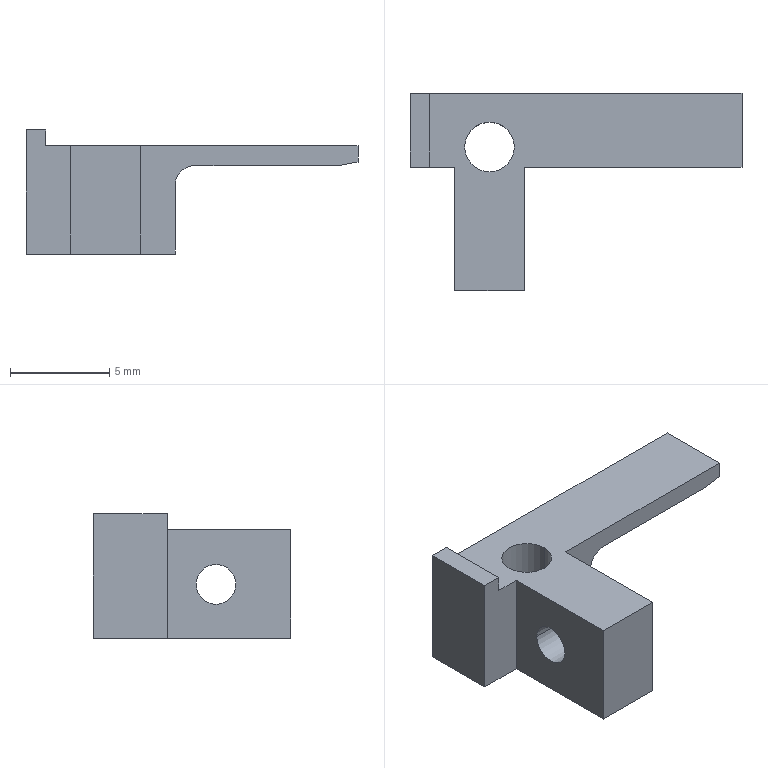Part | NX | 1 solid | 23 faces | box 16.7 x 9.913 x 6.24 mm | volume 257.778 mm3 | plane 16 | cylinder 7 | commonest cylinder face diameters 2 x3 2.5 x2 3.1 x2
STEP:
#1=CARTESIAN_POINT('',(-38.91,-45.316,4.443));
#2=VERTEX_POINT('',#1);
#3=CARTESIAN_POINT('',(-38.91,-45.316,3.629));
#4=VERTEX_POINT('',#3);
#5=CARTESIAN_POINT('',(-38.91,-45.316,4.403));
#6=DIRECTION('',(0.,0.,-1.));
#7=VECTOR('',#6,1000.);
#8=LINE('',#5,#7);
#9=EDGE_CURVE('',#2,#4,#8,.T.);
#10=ORIENTED_EDGE('',*,*,#9,.T.);
#11=CARTESIAN_POINT('',(-39.91,-45.316,3.453));
#12=VERTEX_POINT('',#11);
#13=CARTESIAN_POINT('',(-49.101,-45.316,1.833));
#14=DIRECTION('',(0.9848,0.,0.1736));
#15=VECTOR('',#14,1000.);
#16=LINE('',#13,#15);
#17=EDGE_CURVE('',#12,#4,#16,.T.);
#18=ORIENTED_EDGE('',*,*,#17,.F.);
#19=CARTESIAN_POINT('',(-47.11,-45.316,3.453));
#20=VERTEX_POINT('',#19);
#21=CARTESIAN_POINT('',(-49.101,-45.316,3.453));
#22=DIRECTION('',(-1.,0.,0.));
#23=VECTOR('',#22,1000.);
#24=LINE('',#21,#23);
#25=EDGE_CURVE('',#12,#20,#24,.T.);
#26=ORIENTED_EDGE('',*,*,#25,.T.);
#27=CARTESIAN_POINT('',(-48.11,-45.316,2.453));
#28=VERTEX_POINT('',#27);
#29=CARTESIAN_POINT('',(-47.11,-45.316,2.453));
#30=DIRECTION('',(0.,1.,0.));
#31=DIRECTION('',(0.,0.,1.));
#32=AXIS2_PLACEMENT_3D('',#29,#30,#31);
#33=CIRCLE('',#32,1.);
#34=EDGE_CURVE('',#28,#20,#33,.T.);
#35=ORIENTED_EDGE('',*,*,#34,.F.);
#36=CARTESIAN_POINT('',(-48.11,-45.316,-0.9969));
#37=VERTEX_POINT('',#36);
#38=CARTESIAN_POINT('',(-48.11,-45.316,4.403));
#39=DIRECTION('',(0.,0.,-1.));
#40=VECTOR('',#39,1000.);
#41=LINE('',#38,#40);
#42=EDGE_CURVE('',#28,#37,#41,.T.);
#43=ORIENTED_EDGE('',*,*,#42,.T.);
#44=CARTESIAN_POINT('',(-55.61,-45.316,-0.9969));
#45=VERTEX_POINT('',#44);
#46=CARTESIAN_POINT('',(-49.101,-45.316,-0.9969));
#47=DIRECTION('',(-1.,0.,0.));
#48=VECTOR('',#47,1000.);
#49=LINE('',#46,#48);
#50=EDGE_CURVE('',#37,#45,#49,.T.);
#51=ORIENTED_EDGE('',*,*,#50,.T.);
#52=CARTESIAN_POINT('',(-55.61,-45.316,5.243));
#53=VERTEX_POINT('',#52);
#54=CARTESIAN_POINT('',(-55.61,-45.316,4.403));
#55=DIRECTION('',(0.,0.,1.));
#56=VECTOR('',#55,1000.);
#57=LINE('',#54,#56);
#58=EDGE_CURVE('',#45,#53,#57,.T.);
#59=ORIENTED_EDGE('',*,*,#58,.T.);
#60=CARTESIAN_POINT('',(-54.61,-45.316,5.243));
#61=VERTEX_POINT('',#60);
#62=CARTESIAN_POINT('',(-49.101,-45.316,5.243));
#63=DIRECTION('',(1.,0.,0.));
#64=VECTOR('',#63,1000.);
#65=LINE('',#62,#64);
#66=EDGE_CURVE('',#53,#61,#65,.T.);
#67=ORIENTED_EDGE('',*,*,#66,.T.);
#68=CARTESIAN_POINT('',(-54.61,-45.316,4.443));
#69=VERTEX_POINT('',#68);
#70=CARTESIAN_POINT('',(-54.61,-45.316,4.403));
#71=DIRECTION('',(0.,0.,1.));
#72=VECTOR('',#71,1000.);
#73=LINE('',#70,#72);
#74=EDGE_CURVE('',#69,#61,#73,.T.);
#75=ORIENTED_EDGE('',*,*,#74,.F.);
#76=CARTESIAN_POINT('',(-49.101,-45.316,4.443));
#77=DIRECTION('',(1.,0.,0.));
#78=VECTOR('',#77,1000.);
#79=LINE('',#76,#78);
#80=EDGE_CURVE('',#69,#2,#79,.T.);
#81=ORIENTED_EDGE('',*,*,#80,.T.);
#82=EDGE_LOOP('',(#10,#18,#26,#35,#43,#51,#59,#67,#75,#81));
#83=FACE_BOUND('',#82,.T.);
#84=CARTESIAN_POINT('',(-43.64,-45.316,3.458));
#85=DIRECTION('',(0.,1.,0.));
#86=DIRECTION('',(1.,0.,0.));
#87=AXIS2_PLACEMENT_3D('',#84,#85,#86);
#88=PLANE('',#87);
#89=ADVANCED_FACE('',(#83),#88,.T.);
#90=CARTESIAN_POINT('',(-54.61,-49.029,5.243));
#91=VERTEX_POINT('',#90);
#92=CARTESIAN_POINT('',(-54.61,-49.029,4.443));
#93=VERTEX_POINT('',#92);
#94=CARTESIAN_POINT('',(-54.61,-49.029,4.403));
#95=DIRECTION('',(0.,0.,-1.));
#96=VECTOR('',#95,1000.);
#97=LINE('',#94,#96);
#98=EDGE_CURVE('',#91,#93,#97,.T.);
#99=ORIENTED_EDGE('',*,*,#98,.F.);
#100=CARTESIAN_POINT('',(-55.61,-49.029,5.243));
#101=VERTEX_POINT('',#100);
#102=CARTESIAN_POINT('',(-49.101,-49.029,5.243));
#103=DIRECTION('',(-1.,0.,0.));
#104=VECTOR('',#103,1000.);
#105=LINE('',#102,#104);
#106=EDGE_CURVE('',#91,#101,#105,.T.);
#107=ORIENTED_EDGE('',*,*,#106,.T.);
#108=CARTESIAN_POINT('',(-55.61,-49.029,-0.9969));
#109=VERTEX_POINT('',#108);
#110=CARTESIAN_POINT('',(-55.61,-49.029,4.403));
#111=DIRECTION('',(0.,0.,1.));
#112=VECTOR('',#111,1000.);
#113=LINE('',#110,#112);
#114=EDGE_CURVE('',#109,#101,#113,.T.);
#115=ORIENTED_EDGE('',*,*,#114,.F.);
#116=CARTESIAN_POINT('',(-53.36,-49.029,-0.9969));
#117=VERTEX_POINT('',#116);
#118=CARTESIAN_POINT('',(-49.101,-49.029,-0.9969));
#119=DIRECTION('',(-1.,0.,0.));
#120=VECTOR('',#119,1000.);
#121=LINE('',#118,#120);
#122=EDGE_CURVE('',#117,#109,#121,.T.);
#123=ORIENTED_EDGE('',*,*,#122,.F.);
#124=CARTESIAN_POINT('',(-53.36,-49.029,4.443));
#125=VERTEX_POINT('',#124);
#126=CARTESIAN_POINT('',(-53.36,-49.029,4.403));
#127=DIRECTION('',(0.,0.,1.));
#128=VECTOR('',#127,1000.);
#129=LINE('',#126,#128);
#130=EDGE_CURVE('',#117,#125,#129,.T.);
#131=ORIENTED_EDGE('',*,*,#130,.T.);
#132=CARTESIAN_POINT('',(-49.101,-49.029,4.443));
#133=DIRECTION('',(-1.,0.,0.));
#134=VECTOR('',#133,1000.);
#135=LINE('',#132,#134);
#136=EDGE_CURVE('',#125,#93,#135,.T.);
#137=ORIENTED_EDGE('',*,*,#136,.T.);
#138=EDGE_LOOP('',(#99,#107,#115,#123,#131,#137));
#139=FACE_BOUND('',#138,.T.);
#140=CARTESIAN_POINT('',(-54.61,-49.029,4.403));
#141=DIRECTION('',(0.,-1.,0.));
#142=DIRECTION('',(0.,0.,-1.));
#143=AXIS2_PLACEMENT_3D('',#140,#141,#142);
#144=PLANE('',#143);
#145=ADVANCED_FACE('',(#139),#144,.T.);
#146=CARTESIAN_POINT('',(-48.11,-49.029,2.453));
#147=VERTEX_POINT('',#146);
#148=CARTESIAN_POINT('',(-48.11,-51.163,2.453));
#149=DIRECTION('',(0.,1.,0.));
#150=VECTOR('',#149,1000.);
#151=LINE('',#148,#150);
#152=EDGE_CURVE('',#147,#28,#151,.T.);
#153=ORIENTED_EDGE('',*,*,#152,.F.);
#154=CARTESIAN_POINT('',(-48.11,-49.029,-0.9969));
#155=VERTEX_POINT('',#154);
#156=CARTESIAN_POINT('',(-48.11,-49.029,4.403));
#157=DIRECTION('',(0.,0.,1.));
#158=VECTOR('',#157,1000.);
#159=LINE('',#156,#158);
#160=EDGE_CURVE('',#155,#147,#159,.T.);
#161=ORIENTED_EDGE('',*,*,#160,.F.);
#162=CARTESIAN_POINT('',(-48.11,-51.163,-0.9969));
#163=DIRECTION('',(0.,-1.,0.));
#164=VECTOR('',#163,1000.);
#165=LINE('',#162,#164);
#166=EDGE_CURVE('',#37,#155,#165,.T.);
#167=ORIENTED_EDGE('',*,*,#166,.F.);
#168=ORIENTED_EDGE('',*,*,#42,.F.);
#169=EDGE_LOOP('',(#153,#161,#167,#168));
#170=FACE_BOUND('',#169,.T.);
#171=CARTESIAN_POINT('',(-48.11,-47.529,-0.5969));
#172=DIRECTION('',(1.,0.,0.));
#173=DIRECTION('',(0.,1.,0.));
#174=AXIS2_PLACEMENT_3D('',#171,#172,#173);
#175=PLANE('',#174);
#176=ADVANCED_FACE('',(#170),#175,.T.);
#177=CARTESIAN_POINT('',(-55.61,-51.163,5.243));
#178=DIRECTION('',(0.,1.,0.));
#179=VECTOR('',#178,1000.);
#180=LINE('',#177,#179);
#181=EDGE_CURVE('',#101,#53,#180,.T.);
#182=ORIENTED_EDGE('',*,*,#181,.F.);
#183=ORIENTED_EDGE('',*,*,#106,.F.);
#184=CARTESIAN_POINT('',(-54.61,-51.163,5.243));
#185=DIRECTION('',(0.,-1.,0.));
#186=VECTOR('',#185,1000.);
#187=LINE('',#184,#186);
#188=EDGE_CURVE('',#61,#91,#187,.T.);
#189=ORIENTED_EDGE('',*,*,#188,.F.);
#190=ORIENTED_EDGE('',*,*,#66,.F.);
#191=EDGE_LOOP('',(#182,#183,#189,#190));
#192=FACE_BOUND('',#191,.T.);
#193=CARTESIAN_POINT('',(-55.143,-49.311,5.243));
#194=DIRECTION('',(0.,0.,1.));
#195=DIRECTION('',(1.,0.,0.));
#196=AXIS2_PLACEMENT_3D('',#193,#194,#195);
#197=PLANE('',#196);
#198=ADVANCED_FACE('',(#192),#197,.T.);
#199=ORIENTED_EDGE('',*,*,#114,.T.);
#200=ORIENTED_EDGE('',*,*,#181,.T.);
#201=ORIENTED_EDGE('',*,*,#58,.F.);
#202=CARTESIAN_POINT('',(-55.61,-51.163,-0.9969));
#203=DIRECTION('',(0.,1.,0.));
#204=VECTOR('',#203,1000.);
#205=LINE('',#202,#204);
#206=EDGE_CURVE('',#109,#45,#205,.T.);
#207=ORIENTED_EDGE('',*,*,#206,.F.);
#208=EDGE_LOOP('',(#199,#200,#201,#207));
#209=FACE_BOUND('',#208,.T.);
#210=CARTESIAN_POINT('',(-55.61,-49.729,4.403));
#211=DIRECTION('',(-1.,0.,0.));
#212=DIRECTION('',(0.,0.,1.));
#213=AXIS2_PLACEMENT_3D('',#210,#211,#212);
#214=PLANE('',#213);
#215=ADVANCED_FACE('',(#209),#214,.T.);
#216=CARTESIAN_POINT('',(-54.61,-51.163,4.443));
#217=DIRECTION('',(0.,-1.,0.));
#218=VECTOR('',#217,1000.);
#219=LINE('',#216,#218);
#220=EDGE_CURVE('',#69,#93,#219,.T.);
#221=ORIENTED_EDGE('',*,*,#220,.F.);
#222=ORIENTED_EDGE('',*,*,#74,.T.);
#223=ORIENTED_EDGE('',*,*,#188,.T.);
#224=ORIENTED_EDGE('',*,*,#98,.T.);
#225=EDGE_LOOP('',(#221,#222,#223,#224));
#226=FACE_BOUND('',#225,.T.);
#227=CARTESIAN_POINT('',(-54.61,-45.316,4.403));
#228=DIRECTION('',(1.,0.,0.));
#229=DIRECTION('',(0.,1.,0.));
#230=AXIS2_PLACEMENT_3D('',#227,#228,#229);
#231=PLANE('',#230);
#232=ADVANCED_FACE('',(#226),#231,.T.);
#233=CARTESIAN_POINT('',(-38.91,-49.029,4.443));
#234=VERTEX_POINT('',#233);
#235=CARTESIAN_POINT('',(-38.91,-51.163,4.443));
#236=DIRECTION('',(0.,-1.,0.));
#237=VECTOR('',#236,1000.);
#238=LINE('',#235,#237);
#239=EDGE_CURVE('',#2,#234,#238,.T.);
#240=ORIENTED_EDGE('',*,*,#239,.F.);
#241=ORIENTED_EDGE('',*,*,#80,.F.);
#242=ORIENTED_EDGE('',*,*,#220,.T.);
#243=ORIENTED_EDGE('',*,*,#136,.F.);
#244=CARTESIAN_POINT('',(-53.36,-55.229,4.443));
#245=VERTEX_POINT('',#244);
#246=CARTESIAN_POINT('',(-53.36,-51.163,4.443));
#247=DIRECTION('',(0.,1.,0.));
#248=VECTOR('',#247,1000.);
#249=LINE('',#246,#248);
#250=EDGE_CURVE('',#245,#125,#249,.T.);
#251=ORIENTED_EDGE('',*,*,#250,.F.);
#252=CARTESIAN_POINT('',(-49.86,-55.229,4.443));
#253=VERTEX_POINT('',#252);
#254=CARTESIAN_POINT('',(-49.101,-55.229,4.443));
#255=DIRECTION('',(-1.,0.,0.));
#256=VECTOR('',#255,1000.);
#257=LINE('',#254,#256);
#258=EDGE_CURVE('',#253,#245,#257,.T.);
#259=ORIENTED_EDGE('',*,*,#258,.F.);
#260=CARTESIAN_POINT('',(-49.86,-49.029,4.443));
#261=VERTEX_POINT('',#260);
#262=CARTESIAN_POINT('',(-49.86,-51.163,4.443));
#263=DIRECTION('',(0.,-1.,0.));
#264=VECTOR('',#263,1000.);
#265=LINE('',#262,#264);
#266=EDGE_CURVE('',#261,#253,#265,.T.);
#267=ORIENTED_EDGE('',*,*,#266,.F.);
#268=CARTESIAN_POINT('',(-49.101,-49.029,4.443));
#269=DIRECTION('',(-1.,0.,0.));
#270=VECTOR('',#269,1000.);
#271=LINE('',#268,#270);
#272=EDGE_CURVE('',#234,#261,#271,.T.);
#273=ORIENTED_EDGE('',*,*,#272,.F.);
#274=EDGE_LOOP('',(#240,#241,#242,#243,#251,#259,#267,#273));
#275=FACE_BOUND('',#274,.T.);
#276=CARTESIAN_POINT('',(-50.36,-48.012,4.443));
#277=VERTEX_POINT('',#276);
#278=CARTESIAN_POINT('',(-52.86,-48.012,4.443));
#279=VERTEX_POINT('',#278);
#280=CARTESIAN_POINT('',(-51.61,-48.012,4.443));
#281=DIRECTION('',(0.,0.,-1.));
#282=DIRECTION('',(-1.,0.,0.));
#283=AXIS2_PLACEMENT_3D('',#280,#281,#282);
#284=CIRCLE('',#283,1.25);
#285=EDGE_CURVE('',#277,#279,#284,.T.);
#286=ORIENTED_EDGE('',*,*,#285,.T.);
#287=CARTESIAN_POINT('',(-51.61,-48.012,4.443));
#288=DIRECTION('',(0.,0.,-1.));
#289=DIRECTION('',(-1.,0.,0.));
#290=AXIS2_PLACEMENT_3D('',#287,#288,#289);
#291=CIRCLE('',#290,1.25);
#292=EDGE_CURVE('',#279,#277,#291,.T.);
#293=ORIENTED_EDGE('',*,*,#292,.T.);
#294=EDGE_LOOP('',(#286,#293));
#295=FACE_BOUND('',#294,.T.);
#296=CARTESIAN_POINT('',(-39.41,-47.687,4.443));
#297=DIRECTION('',(0.,0.,1.));
#298=DIRECTION('',(1.,0.,0.));
#299=AXIS2_PLACEMENT_3D('',#296,#297,#298);
#300=PLANE('',#299);
#301=ADVANCED_FACE('',(#275,#295),#300,.T.);
#302=CARTESIAN_POINT('',(-47.11,-49.029,3.453));
#303=VERTEX_POINT('',#302);
#304=CARTESIAN_POINT('',(-39.91,-49.029,3.453));
#305=VERTEX_POINT('',#304);
#306=CARTESIAN_POINT('',(-49.101,-49.029,3.453));
#307=DIRECTION('',(1.,0.,0.));
#308=VECTOR('',#307,1000.);
#309=LINE('',#306,#308);
#310=EDGE_CURVE('',#303,#305,#309,.T.);
#311=ORIENTED_EDGE('',*,*,#310,.F.);
#312=CARTESIAN_POINT('',(-47.11,-51.163,3.453));
#313=DIRECTION('',(0.,1.,0.));
#314=VECTOR('',#313,1000.);
#315=LINE('',#312,#314);
#316=EDGE_CURVE('',#303,#20,#315,.T.);
#317=ORIENTED_EDGE('',*,*,#316,.T.);
#318=ORIENTED_EDGE('',*,*,#25,.F.);
#319=CARTESIAN_POINT('',(-39.91,-47.172,3.453));
#320=DIRECTION('',(0.,1.,0.));
#321=VECTOR('',#320,1000.);
#322=LINE('',#319,#321);
#323=EDGE_CURVE('',#305,#12,#322,.T.);
#324=ORIENTED_EDGE('',*,*,#323,.F.);
#325=EDGE_LOOP('',(#311,#317,#318,#324));
#326=FACE_BOUND('',#325,.T.);
#327=CARTESIAN_POINT('',(-41.41,-56.22,3.453));
#328=DIRECTION('',(0.,0.,1.));
#329=DIRECTION('',(1.,0.,0.));
#330=AXIS2_PLACEMENT_3D('',#327,#328,#329);
#331=PLANE('',#330);
#332=ADVANCED_FACE('',(#326),#331,.F.);
#333=ORIENTED_EDGE('',*,*,#152,.T.);
#334=ORIENTED_EDGE('',*,*,#34,.T.);
#335=ORIENTED_EDGE('',*,*,#316,.F.);
#336=CARTESIAN_POINT('',(-47.11,-49.029,2.453));
#337=DIRECTION('',(0.,1.,0.));
#338=DIRECTION('',(0.,0.,1.));
#339=AXIS2_PLACEMENT_3D('',#336,#337,#338);
#340=CIRCLE('',#339,1.);
#341=EDGE_CURVE('',#147,#303,#340,.T.);
#342=ORIENTED_EDGE('',*,*,#341,.F.);
#343=EDGE_LOOP('',(#333,#334,#335,#342));
#344=FACE_BOUND('',#343,.T.);
#345=CARTESIAN_POINT('',(-47.11,-51.163,2.453));
#346=DIRECTION('',(0.,1.,0.));
#347=DIRECTION('',(0.,0.,1.));
#348=AXIS2_PLACEMENT_3D('',#345,#346,#347);
#349=CYLINDRICAL_SURFACE('',#348,1.);
#350=ADVANCED_FACE('',(#344),#349,.F.);
#351=CARTESIAN_POINT('',(-50.06,-53.51,0.5031));
#352=VERTEX_POINT('',#351);
#353=CARTESIAN_POINT('',(-53.16,-53.51,0.5031));
#354=VERTEX_POINT('',#353);
#355=CARTESIAN_POINT('',(-51.61,-53.51,0.5031));
#356=DIRECTION('',(0.,0.,-1.));
#357=DIRECTION('',(-1.,0.,0.));
#358=AXIS2_PLACEMENT_3D('',#355,#356,#357);
#359=CIRCLE('',#358,1.55);
#360=EDGE_CURVE('',#352,#354,#359,.T.);
#361=ORIENTED_EDGE('',*,*,#360,.T.);
#362=CARTESIAN_POINT('',(-51.61,-53.51,0.5031));
#363=DIRECTION('',(0.,0.,-1.));
#364=DIRECTION('',(-1.,0.,0.));
#365=AXIS2_PLACEMENT_3D('',#362,#363,#364);
#366=CIRCLE('',#365,1.55);
#367=EDGE_CURVE('',#354,#352,#366,.T.);
#368=ORIENTED_EDGE('',*,*,#367,.T.);
#369=EDGE_LOOP('',(#361,#368));
#370=FACE_BOUND('',#369,.T.);
#371=CARTESIAN_POINT('',(-51.111,-53.01,0.5031));
#372=DIRECTION('',(0.,0.,-1.));
#373=DIRECTION('',(0.,-1.,0.));
#374=AXIS2_PLACEMENT_3D('',#371,#372,#373);
#375=PLANE('',#374);
#376=ADVANCED_FACE('',(#370),#375,.T.);
#377=CARTESIAN_POINT('',(-50.36,-48.012,-0.9969));
#378=VERTEX_POINT('',#377);
#379=CARTESIAN_POINT('',(-52.86,-48.012,-0.9969));
#380=VERTEX_POINT('',#379);
#381=CARTESIAN_POINT('',(-51.61,-48.012,-0.9969));
#382=DIRECTION('',(0.,0.,-1.));
#383=DIRECTION('',(-1.,0.,0.));
#384=AXIS2_PLACEMENT_3D('',#381,#382,#383);
#385=CIRCLE('',#384,1.25);
#386=EDGE_CURVE('',#378,#380,#385,.T.);
#387=ORIENTED_EDGE('',*,*,#386,.T.);
#388=CARTESIAN_POINT('',(-52.86,-48.012,-2.597));
#389=DIRECTION('',(0.,0.,-1.));
#390=VECTOR('',#389,1000.);
#391=LINE('',#388,#390);
#392=EDGE_CURVE('',#380,#279,#391,.F.);
#393=ORIENTED_EDGE('',*,*,#392,.T.);
#394=ORIENTED_EDGE('',*,*,#285,.F.);
#395=CARTESIAN_POINT('',(-50.36,-48.012,-2.597));
#396=DIRECTION('',(0.,0.,-1.));
#397=VECTOR('',#396,1000.);
#398=LINE('',#395,#397);
#399=EDGE_CURVE('',#378,#277,#398,.F.);
#400=ORIENTED_EDGE('',*,*,#399,.F.);
#401=EDGE_LOOP('',(#387,#393,#394,#400));
#402=FACE_BOUND('',#401,.T.);
#403=CARTESIAN_POINT('',(-51.61,-48.012,-2.597));
#404=DIRECTION('',(0.,0.,-1.));
#405=DIRECTION('',(-1.,0.,0.));
#406=AXIS2_PLACEMENT_3D('',#403,#404,#405);
#407=CYLINDRICAL_SURFACE('',#406,1.25);
#408=ADVANCED_FACE('',(#402),#407,.F.);
#409=ORIENTED_EDGE('',*,*,#310,.T.);
#410=CARTESIAN_POINT('',(-38.91,-49.029,3.629));
#411=VERTEX_POINT('',#410);
#412=CARTESIAN_POINT('',(-49.101,-49.029,1.833));
#413=DIRECTION('',(-0.9848,0.,-0.1736));
#414=VECTOR('',#413,1000.);
#415=LINE('',#412,#414);
#416=EDGE_CURVE('',#411,#305,#415,.T.);
#417=ORIENTED_EDGE('',*,*,#416,.F.);
#418=CARTESIAN_POINT('',(-38.91,-49.029,4.403));
#419=DIRECTION('',(0.,0.,1.));
#420=VECTOR('',#419,1000.);
#421=LINE('',#418,#420);
#422=EDGE_CURVE('',#411,#234,#421,.T.);
#423=ORIENTED_EDGE('',*,*,#422,.T.);
#424=ORIENTED_EDGE('',*,*,#272,.T.);
#425=CARTESIAN_POINT('',(-49.86,-49.029,-0.9969));
#426=VERTEX_POINT('',#425);
#427=CARTESIAN_POINT('',(-49.86,-49.029,4.403));
#428=DIRECTION('',(0.,0.,-1.));
#429=VECTOR('',#428,1000.);
#430=LINE('',#427,#429);
#431=EDGE_CURVE('',#261,#426,#430,.T.);
#432=ORIENTED_EDGE('',*,*,#431,.T.);
#433=CARTESIAN_POINT('',(-49.101,-49.029,-0.9969));
#434=DIRECTION('',(-1.,0.,0.));
#435=VECTOR('',#434,1000.);
#436=LINE('',#433,#435);
#437=EDGE_CURVE('',#155,#426,#436,.T.);
#438=ORIENTED_EDGE('',*,*,#437,.F.);
#439=ORIENTED_EDGE('',*,*,#160,.T.);
#440=ORIENTED_EDGE('',*,*,#341,.T.);
#441=EDGE_LOOP('',(#409,#417,#423,#424,#432,#438,#439,#440));
#442=FACE_BOUND('',#441,.T.);
#443=CARTESIAN_POINT('',(-41.41,-49.029,3.403));
#444=DIRECTION('',(0.,-1.,0.));
#445=DIRECTION('',(0.,0.,-1.));
#446=AXIS2_PLACEMENT_3D('',#443,#444,#445);
#447=PLANE('',#446);
#448=ADVANCED_FACE('',(#442),#447,.T.);
#449=CARTESIAN_POINT('',(-50.06,-53.51,-0.9969));
#450=VERTEX_POINT('',#449);
#451=CARTESIAN_POINT('',(-53.16,-53.51,-0.9969));
#452=VERTEX_POINT('',#451);
#453=CARTESIAN_POINT('',(-51.61,-53.51,-0.9969));
#454=DIRECTION('',(0.,0.,-1.));
#455=DIRECTION('',(-1.,0.,0.));
#456=AXIS2_PLACEMENT_3D('',#453,#454,#455);
#457=CIRCLE('',#456,1.55);
#458=EDGE_CURVE('',#450,#452,#457,.T.);
#459=ORIENTED_EDGE('',*,*,#458,.T.);
#460=CARTESIAN_POINT('',(-53.16,-53.51,-0.9969));
#461=DIRECTION('',(0.,0.,-1.));
#462=VECTOR('',#461,1000.);
#463=LINE('',#460,#462);
#464=EDGE_CURVE('',#452,#354,#463,.F.);
#465=ORIENTED_EDGE('',*,*,#464,.T.);
#466=ORIENTED_EDGE('',*,*,#360,.F.);
#467=CARTESIAN_POINT('',(-50.06,-53.51,-0.9969));
#468=DIRECTION('',(0.,0.,-1.));
#469=VECTOR('',#468,1000.);
#470=LINE('',#467,#469);
#471=EDGE_CURVE('',#450,#352,#470,.F.);
#472=ORIENTED_EDGE('',*,*,#471,.F.);
#473=EDGE_LOOP('',(#459,#465,#466,#472));
#474=FACE_BOUND('',#473,.T.);
#475=CARTESIAN_POINT('',(-51.61,-53.51,-0.9969));
#476=DIRECTION('',(0.,0.,-1.));
#477=DIRECTION('',(-1.,0.,0.));
#478=AXIS2_PLACEMENT_3D('',#475,#476,#477);
#479=CYLINDRICAL_SURFACE('',#478,1.55);
#480=ADVANCED_FACE('',(#474),#479,.F.);
#481=CARTESIAN_POINT('',(-53.36,-55.229,-0.9969));
#482=VERTEX_POINT('',#481);
#483=CARTESIAN_POINT('',(-53.36,-55.229,4.403));
#484=DIRECTION('',(0.,0.,1.));
#485=VECTOR('',#484,1000.);
#486=LINE('',#483,#485);
#487=EDGE_CURVE('',#482,#245,#486,.T.);
#488=ORIENTED_EDGE('',*,*,#487,.F.);
#489=CARTESIAN_POINT('',(-49.86,-55.229,-0.9969));
#490=VERTEX_POINT('',#489);
#491=CARTESIAN_POINT('',(-49.86,-55.229,-0.9969));
#492=DIRECTION('',(-1.,0.,0.));
#493=VECTOR('',#492,1000.);
#494=LINE('',#491,#493);
#495=EDGE_CURVE('',#490,#482,#494,.T.);
#496=ORIENTED_EDGE('',*,*,#495,.F.);
#497=CARTESIAN_POINT('',(-49.86,-55.229,4.403));
#498=DIRECTION('',(0.,0.,-1.));
#499=VECTOR('',#498,1000.);
#500=LINE('',#497,#499);
#501=EDGE_CURVE('',#253,#490,#500,.T.);
#502=ORIENTED_EDGE('',*,*,#501,.F.);
#503=ORIENTED_EDGE('',*,*,#258,.T.);
#504=EDGE_LOOP('',(#488,#496,#502,#503));
#505=FACE_BOUND('',#504,.T.);
#506=CARTESIAN_POINT('',(-51.674,-55.229,-0.05073));
#507=DIRECTION('',(0.,-1.,0.));
#508=DIRECTION('',(0.,0.,-1.));
#509=AXIS2_PLACEMENT_3D('',#506,#507,#508);
#510=PLANE('',#509);
#511=ADVANCED_FACE('',(#505),#510,.T.);
#512=ORIENTED_EDGE('',*,*,#166,.T.);
#513=ORIENTED_EDGE('',*,*,#437,.T.);
#514=CARTESIAN_POINT('',(-49.86,-51.163,-0.9969));
#515=DIRECTION('',(0.,-1.,0.));
#516=VECTOR('',#515,1000.);
#517=LINE('',#514,#516);
#518=EDGE_CURVE('',#426,#490,#517,.T.);
#519=ORIENTED_EDGE('',*,*,#518,.T.);
#520=ORIENTED_EDGE('',*,*,#495,.T.);
#521=CARTESIAN_POINT('',(-53.36,-51.163,-0.9969));
#522=DIRECTION('',(0.,-1.,0.));
#523=VECTOR('',#522,1000.);
#524=LINE('',#521,#523);
#525=EDGE_CURVE('',#117,#482,#524,.T.);
#526=ORIENTED_EDGE('',*,*,#525,.F.);
#527=ORIENTED_EDGE('',*,*,#122,.T.);
#528=ORIENTED_EDGE('',*,*,#206,.T.);
#529=ORIENTED_EDGE('',*,*,#50,.F.);
#530=EDGE_LOOP('',(#512,#513,#519,#520,#526,#527,#528,#529));
#531=FACE_BOUND('',#530,.T.);
#532=ORIENTED_EDGE('',*,*,#458,.F.);
#533=CARTESIAN_POINT('',(-51.61,-53.51,-0.9969));
#534=DIRECTION('',(0.,0.,-1.));
#535=DIRECTION('',(-1.,0.,0.));
#536=AXIS2_PLACEMENT_3D('',#533,#534,#535);
#537=CIRCLE('',#536,1.55);
#538=EDGE_CURVE('',#452,#450,#537,.T.);
#539=ORIENTED_EDGE('',*,*,#538,.F.);
#540=EDGE_LOOP('',(#532,#539));
#541=FACE_BOUND('',#540,.T.);
#542=ORIENTED_EDGE('',*,*,#386,.F.);
#543=CARTESIAN_POINT('',(-51.61,-48.012,-0.9969));
#544=DIRECTION('',(0.,0.,-1.));
#545=DIRECTION('',(-1.,0.,0.));
#546=AXIS2_PLACEMENT_3D('',#543,#544,#545);
#547=CIRCLE('',#546,1.25);
#548=EDGE_CURVE('',#380,#378,#547,.T.);
#549=ORIENTED_EDGE('',*,*,#548,.F.);
#550=EDGE_LOOP('',(#542,#549));
#551=FACE_BOUND('',#550,.T.);
#552=CARTESIAN_POINT('',(-49.101,-51.163,-0.9969));
#553=DIRECTION('',(0.,0.,-1.));
#554=DIRECTION('',(0.,-1.,0.));
#555=AXIS2_PLACEMENT_3D('',#552,#553,#554);
#556=PLANE('',#555);
#557=ADVANCED_FACE('',(#531,#541,#551),#556,.T.);
#558=CARTESIAN_POINT('',(-49.86,-50.479,1.703));
#559=VERTEX_POINT('',#558);
#560=CARTESIAN_POINT('',(-49.86,-52.479,1.703));
#561=VERTEX_POINT('',#560);
#562=CARTESIAN_POINT('',(-49.86,-51.479,1.703));
#563=DIRECTION('',(-1.,0.,0.));
#564=DIRECTION('',(0.,-1.,0.));
#565=AXIS2_PLACEMENT_3D('',#562,#563,#564);
#566=CIRCLE('',#565,1.);
#567=EDGE_CURVE('',#559,#561,#566,.T.);
#568=ORIENTED_EDGE('',*,*,#567,.F.);
#569=CARTESIAN_POINT('',(-53.36,-50.479,1.703));
#570=VERTEX_POINT('',#569);
#571=CARTESIAN_POINT('',(-40.04,-50.479,1.703));
#572=DIRECTION('',(-1.,0.,0.));
#573=VECTOR('',#572,1000.);
#574=LINE('',#571,#573);
#575=EDGE_CURVE('',#570,#559,#574,.F.);
#576=ORIENTED_EDGE('',*,*,#575,.F.);
#577=CARTESIAN_POINT('',(-53.36,-52.479,1.703));
#578=VERTEX_POINT('',#577);
#579=CARTESIAN_POINT('',(-53.36,-51.479,1.703));
#580=DIRECTION('',(-1.,0.,0.));
#581=DIRECTION('',(0.,-1.,0.));
#582=AXIS2_PLACEMENT_3D('',#579,#580,#581);
#583=CIRCLE('',#582,1.);
#584=EDGE_CURVE('',#570,#578,#583,.T.);
#585=ORIENTED_EDGE('',*,*,#584,.T.);
#586=CARTESIAN_POINT('',(-40.04,-52.479,1.703));
#587=DIRECTION('',(-1.,0.,0.));
#588=VECTOR('',#587,1000.);
#589=LINE('',#586,#588);
#590=EDGE_CURVE('',#578,#561,#589,.F.);
#591=ORIENTED_EDGE('',*,*,#590,.T.);
#592=EDGE_LOOP('',(#568,#576,#585,#591));
#593=FACE_BOUND('',#592,.T.);
#594=CARTESIAN_POINT('',(-40.04,-51.479,1.703));
#595=DIRECTION('',(-1.,0.,0.));
#596=DIRECTION('',(0.,-1.,0.));
#597=AXIS2_PLACEMENT_3D('',#594,#595,#596);
#598=CYLINDRICAL_SURFACE('',#597,1.);
#599=ADVANCED_FACE('',(#593),#598,.F.);
#600=ORIENTED_EDGE('',*,*,#431,.F.);
#601=ORIENTED_EDGE('',*,*,#266,.T.);
#602=ORIENTED_EDGE('',*,*,#501,.T.);
#603=ORIENTED_EDGE('',*,*,#518,.F.);
#604=EDGE_LOOP('',(#600,#601,#602,#603));
#605=FACE_BOUND('',#604,.T.);
#606=ORIENTED_EDGE('',*,*,#567,.T.);
#607=CARTESIAN_POINT('',(-49.86,-51.479,1.703));
#608=DIRECTION('',(-1.,0.,0.));
#609=DIRECTION('',(0.,-1.,0.));
#610=AXIS2_PLACEMENT_3D('',#607,#608,#609);
#611=CIRCLE('',#610,1.);
#612=EDGE_CURVE('',#561,#559,#611,.T.);
#613=ORIENTED_EDGE('',*,*,#612,.T.);
#614=EDGE_LOOP('',(#606,#613));
#615=FACE_BOUND('',#614,.T.);
#616=CARTESIAN_POINT('',(-49.86,-50.229,4.403));
#617=DIRECTION('',(1.,0.,0.));
#618=DIRECTION('',(0.,1.,0.));
#619=AXIS2_PLACEMENT_3D('',#616,#617,#618);
#620=PLANE('',#619);
#621=ADVANCED_FACE('',(#605,#615),#620,.T.);
#622=CARTESIAN_POINT('',(-38.91,-47.172,3.629));
#623=DIRECTION('',(0.,1.,0.));
#624=VECTOR('',#623,1000.);
#625=LINE('',#622,#624);
#626=EDGE_CURVE('',#411,#4,#625,.T.);
#627=ORIENTED_EDGE('',*,*,#626,.T.);
#628=ORIENTED_EDGE('',*,*,#9,.F.);
#629=ORIENTED_EDGE('',*,*,#239,.T.);
#630=ORIENTED_EDGE('',*,*,#422,.F.);
#631=EDGE_LOOP('',(#627,#628,#629,#630));
#632=FACE_BOUND('',#631,.T.);
#633=CARTESIAN_POINT('',(-38.91,-49.283,4.143));
#634=DIRECTION('',(1.,0.,0.));
#635=DIRECTION('',(0.,1.,0.));
#636=AXIS2_PLACEMENT_3D('',#633,#634,#635);
#637=PLANE('',#636);
#638=ADVANCED_FACE('',(#632),#637,.T.);
#639=ORIENTED_EDGE('',*,*,#130,.F.);
#640=ORIENTED_EDGE('',*,*,#525,.T.);
#641=ORIENTED_EDGE('',*,*,#487,.T.);
#642=ORIENTED_EDGE('',*,*,#250,.T.);
#643=EDGE_LOOP('',(#639,#640,#641,#642));
#644=FACE_BOUND('',#643,.T.);
#645=ORIENTED_EDGE('',*,*,#584,.F.);
#646=CARTESIAN_POINT('',(-53.36,-51.479,1.703));
#647=DIRECTION('',(-1.,0.,0.));
#648=DIRECTION('',(0.,-1.,0.));
#649=AXIS2_PLACEMENT_3D('',#646,#647,#648);
#650=CIRCLE('',#649,1.);
#651=EDGE_CURVE('',#578,#570,#650,.T.);
#652=ORIENTED_EDGE('',*,*,#651,.F.);
#653=EDGE_LOOP('',(#645,#652));
#654=FACE_BOUND('',#653,.T.);
#655=CARTESIAN_POINT('',(-53.36,-50.229,-0.9969));
#656=DIRECTION('',(-1.,0.,0.));
#657=DIRECTION('',(0.,0.,1.));
#658=AXIS2_PLACEMENT_3D('',#655,#656,#657);
#659=PLANE('',#658);
#660=ADVANCED_FACE('',(#644,#654),#659,.T.);
#661=ORIENTED_EDGE('',*,*,#626,.F.);
#662=ORIENTED_EDGE('',*,*,#416,.T.);
#663=ORIENTED_EDGE('',*,*,#323,.T.);
#664=ORIENTED_EDGE('',*,*,#17,.T.);
#665=EDGE_LOOP('',(#661,#662,#663,#664));
#666=FACE_BOUND('',#665,.T.);
#667=CARTESIAN_POINT('',(-39.41,-47.172,3.541));
#668=DIRECTION('',(0.1736,0.,-0.9848));
#669=DIRECTION('',(0.,-1.,0.));
#670=AXIS2_PLACEMENT_3D('',#667,#668,#669);
#671=PLANE('',#670);
#672=ADVANCED_FACE('',(#666),#671,.T.);
#673=ORIENTED_EDGE('',*,*,#392,.F.);
#674=ORIENTED_EDGE('',*,*,#548,.T.);
#675=ORIENTED_EDGE('',*,*,#399,.T.);
#676=ORIENTED_EDGE('',*,*,#292,.F.);
#677=EDGE_LOOP('',(#673,#674,#675,#676));
#678=FACE_BOUND('',#677,.T.);
#679=CARTESIAN_POINT('',(-51.61,-48.012,-2.597));
#680=DIRECTION('',(0.,0.,-1.));
#681=DIRECTION('',(-1.,0.,0.));
#682=AXIS2_PLACEMENT_3D('',#679,#680,#681);
#683=CYLINDRICAL_SURFACE('',#682,1.25);
#684=ADVANCED_FACE('',(#678),#683,.F.);
#685=ORIENTED_EDGE('',*,*,#464,.F.);
#686=ORIENTED_EDGE('',*,*,#538,.T.);
#687=ORIENTED_EDGE('',*,*,#471,.T.);
#688=ORIENTED_EDGE('',*,*,#367,.F.);
#689=EDGE_LOOP('',(#685,#686,#687,#688));
#690=FACE_BOUND('',#689,.T.);
#691=CARTESIAN_POINT('',(-51.61,-53.51,-0.9969));
#692=DIRECTION('',(0.,0.,-1.));
#693=DIRECTION('',(-1.,0.,0.));
#694=AXIS2_PLACEMENT_3D('',#691,#692,#693);
#695=CYLINDRICAL_SURFACE('',#694,1.55);
#696=ADVANCED_FACE('',(#690),#695,.F.);
#697=ORIENTED_EDGE('',*,*,#590,.F.);
#698=ORIENTED_EDGE('',*,*,#651,.T.);
#699=ORIENTED_EDGE('',*,*,#575,.T.);
#700=ORIENTED_EDGE('',*,*,#612,.F.);
#701=EDGE_LOOP('',(#697,#698,#699,#700));
#702=FACE_BOUND('',#701,.T.);
#703=CARTESIAN_POINT('',(-40.04,-51.479,1.703));
#704=DIRECTION('',(-1.,0.,0.));
#705=DIRECTION('',(0.,-1.,0.));
#706=AXIS2_PLACEMENT_3D('',#703,#704,#705);
#707=CYLINDRICAL_SURFACE('',#706,1.);
#708=ADVANCED_FACE('',(#702),#707,.F.);
#709=CLOSED_SHELL('',(#89,#145,#176,#198,#215,#232,#301,#332,#350,#376,#408,#448,#480,#511,#557,#599,#621,#638,#660,#672,#684,#696,#708));
#710=MANIFOLD_SOLID_BREP('',#709);
#711=(LENGTH_UNIT()NAMED_UNIT(*)SI_UNIT(.MILLI.,.METRE.));
#712=UNCERTAINTY_MEASURE_WITH_UNIT(LENGTH_MEASURE(0.00001),#711,'','');
#713=(NAMED_UNIT(*)PLANE_ANGLE_UNIT()SI_UNIT($,.RADIAN.));
#714=(NAMED_UNIT(*)SI_UNIT($,.STERADIAN.)SOLID_ANGLE_UNIT());
#715=(GEOMETRIC_REPRESENTATION_CONTEXT(3)GLOBAL_UNCERTAINTY_ASSIGNED_CONTEXT((#712))GLOBAL_UNIT_ASSIGNED_CONTEXT((#711,#713,#714))REPRESENTATION_CONTEXT('',''));
#716=ADVANCED_BREP_SHAPE_REPRESENTATION('',(#710),#715);